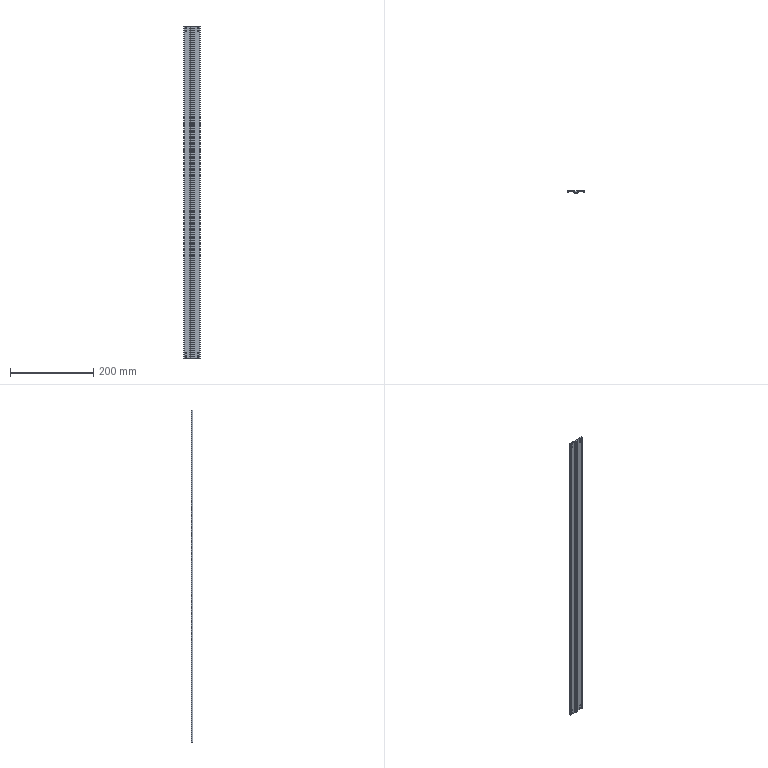Part | STEP file | BODY10_E-RAM6-S-640-ME30-C5 | 1 solid | 38 faces | box 40 x 4.5 x 795.5 mm | volume 67309 mm3 | cylinder 22 | plane 16 | commonest cylinder face diameters 3.4 x8 0.4 x4 0.6 x4 4 x4 2 x2
STEP:
#1=CARTESIAN_POINT('',(-20.,-1.,397.75));
#2=VERTEX_POINT('',#1);
#3=CARTESIAN_POINT('',(-20.,-1.7,397.75));
#4=VERTEX_POINT('',#3);
#5=CARTESIAN_POINT('',(-20.,-2.,397.75));
#6=DIRECTION('',(0.,-1.,0.));
#7=VECTOR('',#6,1000.);
#8=LINE('',#5,#7);
#9=EDGE_CURVE('',#2,#4,#8,.T.);
#10=ORIENTED_EDGE('',*,*,#9,.F.);
#11=CARTESIAN_POINT('',(-20.,-1.,-397.75));
#12=VERTEX_POINT('',#11);
#13=CARTESIAN_POINT('',(-20.,-1.,397.75));
#14=DIRECTION('',(0.,0.,-1.));
#15=VECTOR('',#14,1000.);
#16=LINE('',#13,#15);
#17=EDGE_CURVE('',#2,#12,#16,.T.);
#18=ORIENTED_EDGE('',*,*,#17,.T.);
#19=CARTESIAN_POINT('',(-20.,-1.7,-397.75));
#20=VERTEX_POINT('',#19);
#21=CARTESIAN_POINT('',(-20.,-2.,-397.75));
#22=DIRECTION('',(0.,-1.,0.));
#23=VECTOR('',#22,1000.);
#24=LINE('',#21,#23);
#25=EDGE_CURVE('',#12,#20,#24,.T.);
#26=ORIENTED_EDGE('',*,*,#25,.T.);
#27=CARTESIAN_POINT('',(-20.,-1.7,397.75));
#28=DIRECTION('',(0.,0.,1.));
#29=VECTOR('',#28,1000.);
#30=LINE('',#27,#29);
#31=EDGE_CURVE('',#20,#4,#30,.T.);
#32=ORIENTED_EDGE('',*,*,#31,.T.);
#33=EDGE_LOOP('',(#10,#18,#26,#32));
#34=FACE_OUTER_BOUND('',#33,.T.);
#35=CARTESIAN_POINT('',(-20.,-2.,397.75));
#36=DIRECTION('',(1.,0.,0.));
#37=DIRECTION('',(0.,0.,-1.));
#38=AXIS2_PLACEMENT_3D('',#35,#36,#37);
#39=PLANE('',#38);
#40=ADVANCED_FACE('',(#34),#39,.F.);
#41=CARTESIAN_POINT('',(-19.7,-2.,-397.75));
#42=VERTEX_POINT('',#41);
#43=CARTESIAN_POINT('',(-17.2,-2.,-397.75));
#44=VERTEX_POINT('',#43);
#45=CARTESIAN_POINT('',(-17.,-2.,-397.75));
#46=DIRECTION('',(1.,0.,0.));
#47=VECTOR('',#46,1000.);
#48=LINE('',#45,#47);
#49=EDGE_CURVE('',#42,#44,#48,.T.);
#50=ORIENTED_EDGE('',*,*,#49,.T.);
#51=CARTESIAN_POINT('',(-17.2,-2.,397.75));
#52=VERTEX_POINT('',#51);
#53=CARTESIAN_POINT('',(-17.2,-2.,397.75));
#54=DIRECTION('',(0.,0.,1.));
#55=VECTOR('',#54,1000.);
#56=LINE('',#53,#55);
#57=EDGE_CURVE('',#44,#52,#56,.T.);
#58=ORIENTED_EDGE('',*,*,#57,.T.);
#59=CARTESIAN_POINT('',(-19.7,-2.,397.75));
#60=VERTEX_POINT('',#59);
#61=CARTESIAN_POINT('',(-17.,-2.,397.75));
#62=DIRECTION('',(1.,0.,0.));
#63=VECTOR('',#62,1000.);
#64=LINE('',#61,#63);
#65=EDGE_CURVE('',#60,#52,#64,.T.);
#66=ORIENTED_EDGE('',*,*,#65,.F.);
#67=CARTESIAN_POINT('',(-19.7,-2.,397.75));
#68=DIRECTION('',(0.,0.,-1.));
#69=VECTOR('',#68,1000.);
#70=LINE('',#67,#69);
#71=EDGE_CURVE('',#60,#42,#70,.T.);
#72=ORIENTED_EDGE('',*,*,#71,.T.);
#73=EDGE_LOOP('',(#50,#58,#66,#72));
#74=FACE_OUTER_BOUND('',#73,.T.);
#75=CARTESIAN_POINT('',(-17.,-2.,397.75));
#76=DIRECTION('',(0.,1.,0.));
#77=DIRECTION('',(-1.,0.,0.));
#78=AXIS2_PLACEMENT_3D('',#75,#76,#77);
#79=PLANE('',#78);
#80=ADVANCED_FACE('',(#74),#79,.F.);
#81=CARTESIAN_POINT('',(-17.,-1.8,-397.75));
#82=VERTEX_POINT('',#81);
#83=CARTESIAN_POINT('',(-17.,-1.7,-397.75));
#84=VERTEX_POINT('',#83);
#85=CARTESIAN_POINT('',(-17.,-1.5,-397.75));
#86=DIRECTION('',(0.,1.,0.));
#87=VECTOR('',#86,1000.);
#88=LINE('',#85,#87);
#89=EDGE_CURVE('',#82,#84,#88,.T.);
#90=ORIENTED_EDGE('',*,*,#89,.T.);
#91=CARTESIAN_POINT('',(-17.,-1.7,397.75));
#92=VERTEX_POINT('',#91);
#93=CARTESIAN_POINT('',(-17.,-1.7,397.75));
#94=DIRECTION('',(0.,0.,1.));
#95=VECTOR('',#94,1000.);
#96=LINE('',#93,#95);
#97=EDGE_CURVE('',#84,#92,#96,.T.);
#98=ORIENTED_EDGE('',*,*,#97,.T.);
#99=CARTESIAN_POINT('',(-17.,-1.8,397.75));
#100=VERTEX_POINT('',#99);
#101=CARTESIAN_POINT('',(-17.,-1.5,397.75));
#102=DIRECTION('',(0.,1.,0.));
#103=VECTOR('',#102,1000.);
#104=LINE('',#101,#103);
#105=EDGE_CURVE('',#100,#92,#104,.T.);
#106=ORIENTED_EDGE('',*,*,#105,.F.);
#107=CARTESIAN_POINT('',(-17.,-1.8,397.75));
#108=DIRECTION('',(0.,0.,-1.));
#109=VECTOR('',#108,1000.);
#110=LINE('',#107,#109);
#111=EDGE_CURVE('',#100,#82,#110,.T.);
#112=ORIENTED_EDGE('',*,*,#111,.T.);
#113=EDGE_LOOP('',(#90,#98,#106,#112));
#114=FACE_OUTER_BOUND('',#113,.T.);
#115=CARTESIAN_POINT('',(-17.,-1.5,397.75));
#116=DIRECTION('',(-1.,0.,0.));
#117=DIRECTION('',(0.,0.,1.));
#118=AXIS2_PLACEMENT_3D('',#115,#116,#117);
#119=PLANE('',#118);
#120=ADVANCED_FACE('',(#114),#119,.F.);
#121=CARTESIAN_POINT('',(-16.8,-1.5,397.75));
#122=VERTEX_POINT('',#121);
#123=CARTESIAN_POINT('',(-5.937,-1.5,397.75));
#124=VERTEX_POINT('',#123);
#125=CARTESIAN_POINT('',(-5.,-1.5,397.75));
#126=DIRECTION('',(1.,0.,0.));
#127=VECTOR('',#126,1000.);
#128=LINE('',#125,#127);
#129=EDGE_CURVE('',#122,#124,#128,.T.);
#130=ORIENTED_EDGE('',*,*,#129,.F.);
#131=CARTESIAN_POINT('',(-16.8,-1.5,-397.75));
#132=VERTEX_POINT('',#131);
#133=CARTESIAN_POINT('',(-16.8,-1.5,-397.75));
#134=DIRECTION('',(0.,0.,-1.));
#135=VECTOR('',#134,1000.);
#136=LINE('',#133,#135);
#137=EDGE_CURVE('',#122,#132,#136,.T.);
#138=ORIENTED_EDGE('',*,*,#137,.T.);
#139=CARTESIAN_POINT('',(-5.937,-1.5,-397.75));
#140=VERTEX_POINT('',#139);
#141=CARTESIAN_POINT('',(-5.,-1.5,-397.75));
#142=DIRECTION('',(1.,0.,0.));
#143=VECTOR('',#142,1000.);
#144=LINE('',#141,#143);
#145=EDGE_CURVE('',#132,#140,#144,.T.);
#146=ORIENTED_EDGE('',*,*,#145,.T.);
#147=CARTESIAN_POINT('',(-5.937,-1.5,397.75));
#148=DIRECTION('',(0.,0.,1.));
#149=VECTOR('',#148,1000.);
#150=LINE('',#147,#149);
#151=EDGE_CURVE('',#140,#124,#150,.T.);
#152=ORIENTED_EDGE('',*,*,#151,.T.);
#153=EDGE_LOOP('',(#130,#138,#146,#152));
#154=FACE_OUTER_BOUND('',#153,.T.);
#155=CARTESIAN_POINT('',(-15.7,-1.5,-386.));
#156=VERTEX_POINT('',#155);
#157=CARTESIAN_POINT('',(-14.,-1.5,-387.7));
#158=VERTEX_POINT('',#157);
#159=CARTESIAN_POINT('',(-14.,-1.5,-386.));
#160=DIRECTION('',(0.,-1.,0.));
#161=DIRECTION('',(-1.,0.,0.));
#162=AXIS2_PLACEMENT_3D('',#159,#160,#161);
#163=CIRCLE('',#162,1.7);
#164=EDGE_CURVE('',#156,#158,#163,.T.);
#165=ORIENTED_EDGE('',*,*,#164,.F.);
#166=CARTESIAN_POINT('',(-14.,-1.5,-386.));
#167=DIRECTION('',(0.,-1.,0.));
#168=DIRECTION('',(-1.,0.,0.));
#169=AXIS2_PLACEMENT_3D('',#166,#167,#168);
#170=CIRCLE('',#169,1.7);
#171=EDGE_CURVE('',#158,#156,#170,.T.);
#172=ORIENTED_EDGE('',*,*,#171,.F.);
#173=EDGE_LOOP('',(#165,#172));
#174=FACE_BOUND('',#173,.T.);
#175=CARTESIAN_POINT('',(-15.7,-1.5,-394.));
#176=VERTEX_POINT('',#175);
#177=CARTESIAN_POINT('',(-14.,-1.5,-395.7));
#178=VERTEX_POINT('',#177);
#179=CARTESIAN_POINT('',(-14.,-1.5,-394.));
#180=DIRECTION('',(0.,-1.,0.));
#181=DIRECTION('',(-1.,0.,0.));
#182=AXIS2_PLACEMENT_3D('',#179,#180,#181);
#183=CIRCLE('',#182,1.7);
#184=EDGE_CURVE('',#176,#178,#183,.T.);
#185=ORIENTED_EDGE('',*,*,#184,.F.);
#186=CARTESIAN_POINT('',(-14.,-1.5,-394.));
#187=DIRECTION('',(0.,-1.,0.));
#188=DIRECTION('',(-1.,0.,0.));
#189=AXIS2_PLACEMENT_3D('',#186,#187,#188);
#190=CIRCLE('',#189,1.7);
#191=EDGE_CURVE('',#178,#176,#190,.T.);
#192=ORIENTED_EDGE('',*,*,#191,.F.);
#193=EDGE_LOOP('',(#185,#192));
#194=FACE_BOUND('',#193,.T.);
#195=CARTESIAN_POINT('',(-15.7,-1.5,386.));
#196=VERTEX_POINT('',#195);
#197=CARTESIAN_POINT('',(-14.,-1.5,384.3));
#198=VERTEX_POINT('',#197);
#199=CARTESIAN_POINT('',(-14.,-1.5,386.));
#200=DIRECTION('',(0.,1.,0.));
#201=DIRECTION('',(-1.,0.,0.));
#202=AXIS2_PLACEMENT_3D('',#199,#200,#201);
#203=CIRCLE('',#202,1.7);
#204=EDGE_CURVE('',#196,#198,#203,.T.);
#205=ORIENTED_EDGE('',*,*,#204,.T.);
#206=CARTESIAN_POINT('',(-14.,-1.5,386.));
#207=DIRECTION('',(0.,1.,0.));
#208=DIRECTION('',(-1.,0.,0.));
#209=AXIS2_PLACEMENT_3D('',#206,#207,#208);
#210=CIRCLE('',#209,1.7);
#211=EDGE_CURVE('',#198,#196,#210,.T.);
#212=ORIENTED_EDGE('',*,*,#211,.T.);
#213=EDGE_LOOP('',(#205,#212));
#214=FACE_BOUND('',#213,.T.);
#215=CARTESIAN_POINT('',(-15.7,-1.5,394.));
#216=VERTEX_POINT('',#215);
#217=CARTESIAN_POINT('',(-14.,-1.5,392.3));
#218=VERTEX_POINT('',#217);
#219=CARTESIAN_POINT('',(-14.,-1.5,394.));
#220=DIRECTION('',(0.,1.,0.));
#221=DIRECTION('',(-1.,0.,0.));
#222=AXIS2_PLACEMENT_3D('',#219,#220,#221);
#223=CIRCLE('',#222,1.7);
#224=EDGE_CURVE('',#216,#218,#223,.T.);
#225=ORIENTED_EDGE('',*,*,#224,.T.);
#226=CARTESIAN_POINT('',(-14.,-1.5,394.));
#227=DIRECTION('',(0.,1.,0.));
#228=DIRECTION('',(-1.,0.,0.));
#229=AXIS2_PLACEMENT_3D('',#226,#227,#228);
#230=CIRCLE('',#229,1.7);
#231=EDGE_CURVE('',#218,#216,#230,.T.);
#232=ORIENTED_EDGE('',*,*,#231,.T.);
#233=EDGE_LOOP('',(#225,#232));
#234=FACE_BOUND('',#233,.T.);
#235=CARTESIAN_POINT('',(-5.,-1.5,397.75));
#236=DIRECTION('',(0.,1.,0.));
#237=DIRECTION('',(-1.,0.,0.));
#238=AXIS2_PLACEMENT_3D('',#235,#236,#237);
#239=PLANE('',#238);
#240=ADVANCED_FACE('',(#154,#174,#194,#214,#234),#239,.F.);
#241=CARTESIAN_POINT('',(-4.4,-2.22,-397.75));
#242=VERTEX_POINT('',#241);
#243=CARTESIAN_POINT('',(-3.1,-3.78,-397.75));
#244=VERTEX_POINT('',#243);
#245=CARTESIAN_POINT('',(-2.5,-4.5,-397.75));
#246=DIRECTION('',(0.6402,-0.7682,0.));
#247=VECTOR('',#246,1000.);
#248=LINE('',#245,#247);
#249=EDGE_CURVE('',#242,#244,#248,.T.);
#250=ORIENTED_EDGE('',*,*,#249,.T.);
#251=CARTESIAN_POINT('',(-3.1,-3.78,397.75));
#252=VERTEX_POINT('',#251);
#253=CARTESIAN_POINT('',(-3.1,-3.78,397.75));
#254=DIRECTION('',(0.,0.,1.));
#255=VECTOR('',#254,1000.);
#256=LINE('',#253,#255);
#257=EDGE_CURVE('',#244,#252,#256,.T.);
#258=ORIENTED_EDGE('',*,*,#257,.T.);
#259=CARTESIAN_POINT('',(-4.4,-2.22,397.75));
#260=VERTEX_POINT('',#259);
#261=CARTESIAN_POINT('',(-2.5,-4.5,397.75));
#262=DIRECTION('',(0.6402,-0.7682,0.));
#263=VECTOR('',#262,1000.);
#264=LINE('',#261,#263);
#265=EDGE_CURVE('',#260,#252,#264,.T.);
#266=ORIENTED_EDGE('',*,*,#265,.F.);
#267=CARTESIAN_POINT('',(-4.4,-2.22,-397.75));
#268=DIRECTION('',(0.,0.,-1.));
#269=VECTOR('',#268,1000.);
#270=LINE('',#267,#269);
#271=EDGE_CURVE('',#260,#242,#270,.T.);
#272=ORIENTED_EDGE('',*,*,#271,.T.);
#273=EDGE_LOOP('',(#250,#258,#266,#272));
#274=FACE_OUTER_BOUND('',#273,.T.);
#275=CARTESIAN_POINT('',(-2.5,-4.5,397.75));
#276=DIRECTION('',(0.7682,0.6402,0.));
#277=DIRECTION('',(-0.6402,0.7682,0.));
#278=AXIS2_PLACEMENT_3D('',#275,#276,#277);
#279=PLANE('',#278);
#280=ADVANCED_FACE('',(#274),#279,.F.);
#281=CARTESIAN_POINT('',(-1.563,-4.5,-397.75));
#282=VERTEX_POINT('',#281);
#283=CARTESIAN_POINT('',(1.563,-4.5,-397.75));
#284=VERTEX_POINT('',#283);
#285=CARTESIAN_POINT('',(2.5,-4.5,-397.75));
#286=DIRECTION('',(1.,0.,0.));
#287=VECTOR('',#286,1000.);
#288=LINE('',#285,#287);
#289=EDGE_CURVE('',#282,#284,#288,.T.);
#290=ORIENTED_EDGE('',*,*,#289,.T.);
#291=CARTESIAN_POINT('',(1.563,-4.5,397.75));
#292=VERTEX_POINT('',#291);
#293=CARTESIAN_POINT('',(1.563,-4.5,397.75));
#294=DIRECTION('',(0.,0.,1.));
#295=VECTOR('',#294,1000.);
#296=LINE('',#293,#295);
#297=EDGE_CURVE('',#284,#292,#296,.T.);
#298=ORIENTED_EDGE('',*,*,#297,.T.);
#299=CARTESIAN_POINT('',(-1.563,-4.5,397.75));
#300=VERTEX_POINT('',#299);
#301=CARTESIAN_POINT('',(2.5,-4.5,397.75));
#302=DIRECTION('',(1.,0.,0.));
#303=VECTOR('',#302,1000.);
#304=LINE('',#301,#303);
#305=EDGE_CURVE('',#300,#292,#304,.T.);
#306=ORIENTED_EDGE('',*,*,#305,.F.);
#307=CARTESIAN_POINT('',(-1.563,-4.5,397.75));
#308=DIRECTION('',(0.,0.,-1.));
#309=VECTOR('',#308,1000.);
#310=LINE('',#307,#309);
#311=EDGE_CURVE('',#300,#282,#310,.T.);
#312=ORIENTED_EDGE('',*,*,#311,.T.);
#313=EDGE_LOOP('',(#290,#298,#306,#312));
#314=FACE_OUTER_BOUND('',#313,.T.);
#315=CARTESIAN_POINT('',(2.5,-4.5,397.75));
#316=DIRECTION('',(0.,1.,0.));
#317=DIRECTION('',(0.,0.,1.));
#318=AXIS2_PLACEMENT_3D('',#315,#316,#317);
#319=PLANE('',#318);
#320=ADVANCED_FACE('',(#314),#319,.F.);
#321=CARTESIAN_POINT('',(3.1,-3.78,-397.75));
#322=VERTEX_POINT('',#321);
#323=CARTESIAN_POINT('',(4.4,-2.22,-397.75));
#324=VERTEX_POINT('',#323);
#325=CARTESIAN_POINT('',(5.,-1.5,-397.75));
#326=DIRECTION('',(0.6402,0.7682,0.));
#327=VECTOR('',#326,1000.);
#328=LINE('',#325,#327);
#329=EDGE_CURVE('',#322,#324,#328,.T.);
#330=ORIENTED_EDGE('',*,*,#329,.T.);
#331=CARTESIAN_POINT('',(4.4,-2.22,397.75));
#332=VERTEX_POINT('',#331);
#333=CARTESIAN_POINT('',(4.4,-2.22,397.75));
#334=DIRECTION('',(0.,0.,1.));
#335=VECTOR('',#334,1000.);
#336=LINE('',#333,#335);
#337=EDGE_CURVE('',#324,#332,#336,.T.);
#338=ORIENTED_EDGE('',*,*,#337,.T.);
#339=CARTESIAN_POINT('',(3.1,-3.78,397.75));
#340=VERTEX_POINT('',#339);
#341=CARTESIAN_POINT('',(5.,-1.5,397.75));
#342=DIRECTION('',(0.6402,0.7682,0.));
#343=VECTOR('',#342,1000.);
#344=LINE('',#341,#343);
#345=EDGE_CURVE('',#340,#332,#344,.T.);
#346=ORIENTED_EDGE('',*,*,#345,.F.);
#347=CARTESIAN_POINT('',(3.1,-3.78,397.75));
#348=DIRECTION('',(0.,0.,-1.));
#349=VECTOR('',#348,1000.);
#350=LINE('',#347,#349);
#351=EDGE_CURVE('',#340,#322,#350,.T.);
#352=ORIENTED_EDGE('',*,*,#351,.T.);
#353=EDGE_LOOP('',(#330,#338,#346,#352));
#354=FACE_OUTER_BOUND('',#353,.T.);
#355=CARTESIAN_POINT('',(5.,-1.5,397.75));
#356=DIRECTION('',(-0.7682,0.6402,0.));
#357=DIRECTION('',(-0.6402,-0.7682,0.));
#358=AXIS2_PLACEMENT_3D('',#355,#356,#357);
#359=PLANE('',#358);
#360=ADVANCED_FACE('',(#354),#359,.F.);
#361=CARTESIAN_POINT('',(5.937,-1.5,-397.75));
#362=VERTEX_POINT('',#361);
#363=CARTESIAN_POINT('',(16.8,-1.5,-397.75));
#364=VERTEX_POINT('',#363);
#365=CARTESIAN_POINT('',(17.,-1.5,-397.75));
#366=DIRECTION('',(1.,0.,0.));
#367=VECTOR('',#366,1000.);
#368=LINE('',#365,#367);
#369=EDGE_CURVE('',#362,#364,#368,.T.);
#370=ORIENTED_EDGE('',*,*,#369,.T.);
#371=CARTESIAN_POINT('',(16.8,-1.5,397.75));
#372=VERTEX_POINT('',#371);
#373=CARTESIAN_POINT('',(16.8,-1.5,397.75));
#374=DIRECTION('',(0.,0.,1.));
#375=VECTOR('',#374,1000.);
#376=LINE('',#373,#375);
#377=EDGE_CURVE('',#364,#372,#376,.T.);
#378=ORIENTED_EDGE('',*,*,#377,.T.);
#379=CARTESIAN_POINT('',(5.937,-1.5,397.75));
#380=VERTEX_POINT('',#379);
#381=CARTESIAN_POINT('',(17.,-1.5,397.75));
#382=DIRECTION('',(1.,0.,0.));
#383=VECTOR('',#382,1000.);
#384=LINE('',#381,#383);
#385=EDGE_CURVE('',#380,#372,#384,.T.);
#386=ORIENTED_EDGE('',*,*,#385,.F.);
#387=CARTESIAN_POINT('',(5.937,-1.5,-397.75));
#388=DIRECTION('',(0.,0.,-1.));
#389=VECTOR('',#388,1000.);
#390=LINE('',#387,#389);
#391=EDGE_CURVE('',#380,#362,#390,.T.);
#392=ORIENTED_EDGE('',*,*,#391,.T.);
#393=EDGE_LOOP('',(#370,#378,#386,#392));
#394=FACE_OUTER_BOUND('',#393,.T.);
#395=CARTESIAN_POINT('',(12.3,-1.5,-386.));
#396=VERTEX_POINT('',#395);
#397=CARTESIAN_POINT('',(14.,-1.5,-387.7));
#398=VERTEX_POINT('',#397);
#399=CARTESIAN_POINT('',(14.,-1.5,-386.));
#400=DIRECTION('',(0.,-1.,0.));
#401=DIRECTION('',(-1.,0.,0.));
#402=AXIS2_PLACEMENT_3D('',#399,#400,#401);
#403=CIRCLE('',#402,1.7);
#404=EDGE_CURVE('',#396,#398,#403,.T.);
#405=ORIENTED_EDGE('',*,*,#404,.F.);
#406=CARTESIAN_POINT('',(14.,-1.5,-386.));
#407=DIRECTION('',(0.,-1.,0.));
#408=DIRECTION('',(-1.,0.,0.));
#409=AXIS2_PLACEMENT_3D('',#406,#407,#408);
#410=CIRCLE('',#409,1.7);
#411=EDGE_CURVE('',#398,#396,#410,.T.);
#412=ORIENTED_EDGE('',*,*,#411,.F.);
#413=EDGE_LOOP('',(#405,#412));
#414=FACE_BOUND('',#413,.T.);
#415=CARTESIAN_POINT('',(12.3,-1.5,-394.));
#416=VERTEX_POINT('',#415);
#417=CARTESIAN_POINT('',(14.,-1.5,-395.7));
#418=VERTEX_POINT('',#417);
#419=CARTESIAN_POINT('',(14.,-1.5,-394.));
#420=DIRECTION('',(0.,-1.,0.));
#421=DIRECTION('',(-1.,0.,0.));
#422=AXIS2_PLACEMENT_3D('',#419,#420,#421);
#423=CIRCLE('',#422,1.7);
#424=EDGE_CURVE('',#416,#418,#423,.T.);
#425=ORIENTED_EDGE('',*,*,#424,.F.);
#426=CARTESIAN_POINT('',(14.,-1.5,-394.));
#427=DIRECTION('',(0.,-1.,0.));
#428=DIRECTION('',(-1.,0.,0.));
#429=AXIS2_PLACEMENT_3D('',#426,#427,#428);
#430=CIRCLE('',#429,1.7);
#431=EDGE_CURVE('',#418,#416,#430,.T.);
#432=ORIENTED_EDGE('',*,*,#431,.F.);
#433=EDGE_LOOP('',(#425,#432));
#434=FACE_BOUND('',#433,.T.);
#435=CARTESIAN_POINT('',(12.3,-1.5,386.));
#436=VERTEX_POINT('',#435);
#437=CARTESIAN_POINT('',(14.,-1.5,384.3));
#438=VERTEX_POINT('',#437);
#439=CARTESIAN_POINT('',(14.,-1.5,386.));
#440=DIRECTION('',(0.,1.,0.));
#441=DIRECTION('',(-1.,0.,0.));
#442=AXIS2_PLACEMENT_3D('',#439,#440,#441);
#443=CIRCLE('',#442,1.7);
#444=EDGE_CURVE('',#436,#438,#443,.T.);
#445=ORIENTED_EDGE('',*,*,#444,.T.);
#446=CARTESIAN_POINT('',(14.,-1.5,386.));
#447=DIRECTION('',(0.,1.,0.));
#448=DIRECTION('',(-1.,0.,0.));
#449=AXIS2_PLACEMENT_3D('',#446,#447,#448);
#450=CIRCLE('',#449,1.7);
#451=EDGE_CURVE('',#438,#436,#450,.T.);
#452=ORIENTED_EDGE('',*,*,#451,.T.);
#453=EDGE_LOOP('',(#445,#452));
#454=FACE_BOUND('',#453,.T.);
#455=CARTESIAN_POINT('',(12.3,-1.5,394.));
#456=VERTEX_POINT('',#455);
#457=CARTESIAN_POINT('',(14.,-1.5,392.3));
#458=VERTEX_POINT('',#457);
#459=CARTESIAN_POINT('',(14.,-1.5,394.));
#460=DIRECTION('',(0.,1.,0.));
#461=DIRECTION('',(-1.,0.,0.));
#462=AXIS2_PLACEMENT_3D('',#459,#460,#461);
#463=CIRCLE('',#462,1.7);
#464=EDGE_CURVE('',#456,#458,#463,.T.);
#465=ORIENTED_EDGE('',*,*,#464,.T.);
#466=CARTESIAN_POINT('',(14.,-1.5,394.));
#467=DIRECTION('',(0.,1.,0.));
#468=DIRECTION('',(-1.,0.,0.));
#469=AXIS2_PLACEMENT_3D('',#466,#467,#468);
#470=CIRCLE('',#469,1.7);
#471=EDGE_CURVE('',#458,#456,#470,.T.);
#472=ORIENTED_EDGE('',*,*,#471,.T.);
#473=EDGE_LOOP('',(#465,#472));
#474=FACE_BOUND('',#473,.T.);
#475=CARTESIAN_POINT('',(17.,-1.5,397.75));
#476=DIRECTION('',(0.,1.,0.));
#477=DIRECTION('',(-1.,0.,0.));
#478=AXIS2_PLACEMENT_3D('',#475,#476,#477);
#479=PLANE('',#478);
#480=ADVANCED_FACE('',(#394,#414,#434,#454,#474),#479,.F.);
#481=CARTESIAN_POINT('',(17.,-1.7,397.75));
#482=VERTEX_POINT('',#481);
#483=CARTESIAN_POINT('',(17.,-1.8,397.75));
#484=VERTEX_POINT('',#483);
#485=CARTESIAN_POINT('',(17.,-2.,397.75));
#486=DIRECTION('',(0.,-1.,0.));
#487=VECTOR('',#486,1000.);
#488=LINE('',#485,#487);
#489=EDGE_CURVE('',#482,#484,#488,.T.);
#490=ORIENTED_EDGE('',*,*,#489,.F.);
#491=CARTESIAN_POINT('',(17.,-1.7,-397.75));
#492=VERTEX_POINT('',#491);
#493=CARTESIAN_POINT('',(17.,-1.7,-397.75));
#494=DIRECTION('',(0.,0.,-1.));
#495=VECTOR('',#494,1000.);
#496=LINE('',#493,#495);
#497=EDGE_CURVE('',#482,#492,#496,.T.);
#498=ORIENTED_EDGE('',*,*,#497,.T.);
#499=CARTESIAN_POINT('',(17.,-1.8,-397.75));
#500=VERTEX_POINT('',#499);
#501=CARTESIAN_POINT('',(17.,-2.,-397.75));
#502=DIRECTION('',(0.,-1.,0.));
#503=VECTOR('',#502,1000.);
#504=LINE('',#501,#503);
#505=EDGE_CURVE('',#492,#500,#504,.T.);
#506=ORIENTED_EDGE('',*,*,#505,.T.);
#507=CARTESIAN_POINT('',(17.,-1.8,397.75));
#508=DIRECTION('',(0.,0.,1.));
#509=VECTOR('',#508,1000.);
#510=LINE('',#507,#509);
#511=EDGE_CURVE('',#500,#484,#510,.T.);
#512=ORIENTED_EDGE('',*,*,#511,.T.);
#513=EDGE_LOOP('',(#490,#498,#506,#512));
#514=FACE_OUTER_BOUND('',#513,.T.);
#515=CARTESIAN_POINT('',(17.,-2.,397.75));
#516=DIRECTION('',(1.,0.,0.));
#517=DIRECTION('',(0.,0.,-1.));
#518=AXIS2_PLACEMENT_3D('',#515,#516,#517);
#519=PLANE('',#518);
#520=ADVANCED_FACE('',(#514),#519,.F.);
#521=CARTESIAN_POINT('',(17.2,-2.,397.75));
#522=VERTEX_POINT('',#521);
#523=CARTESIAN_POINT('',(19.7,-2.,397.75));
#524=VERTEX_POINT('',#523);
#525=CARTESIAN_POINT('',(20.,-2.,397.75));
#526=DIRECTION('',(1.,0.,0.));
#527=VECTOR('',#526,1000.);
#528=LINE('',#525,#527);
#529=EDGE_CURVE('',#522,#524,#528,.T.);
#530=ORIENTED_EDGE('',*,*,#529,.F.);
#531=CARTESIAN_POINT('',(17.2,-2.,-397.75));
#532=VERTEX_POINT('',#531);
#533=CARTESIAN_POINT('',(17.2,-2.,397.75));
#534=DIRECTION('',(0.,0.,-1.));
#535=VECTOR('',#534,1000.);
#536=LINE('',#533,#535);
#537=EDGE_CURVE('',#522,#532,#536,.T.);
#538=ORIENTED_EDGE('',*,*,#537,.T.);
#539=CARTESIAN_POINT('',(19.7,-2.,-397.75));
#540=VERTEX_POINT('',#539);
#541=CARTESIAN_POINT('',(20.,-2.,-397.75));
#542=DIRECTION('',(1.,0.,0.));
#543=VECTOR('',#542,1000.);
#544=LINE('',#541,#543);
#545=EDGE_CURVE('',#532,#540,#544,.T.);
#546=ORIENTED_EDGE('',*,*,#545,.T.);
#547=CARTESIAN_POINT('',(19.7,-2.,397.75));
#548=DIRECTION('',(0.,0.,1.));
#549=VECTOR('',#548,1000.);
#550=LINE('',#547,#549);
#551=EDGE_CURVE('',#540,#524,#550,.T.);
#552=ORIENTED_EDGE('',*,*,#551,.T.);
#553=EDGE_LOOP('',(#530,#538,#546,#552));
#554=FACE_OUTER_BOUND('',#553,.T.);
#555=CARTESIAN_POINT('',(20.,-2.,397.75));
#556=DIRECTION('',(0.,1.,0.));
#557=DIRECTION('',(-1.,0.,0.));
#558=AXIS2_PLACEMENT_3D('',#555,#556,#557);
#559=PLANE('',#558);
#560=ADVANCED_FACE('',(#554),#559,.F.);
#561=CARTESIAN_POINT('',(20.,-1.7,-397.75));
#562=VERTEX_POINT('',#561);
#563=CARTESIAN_POINT('',(20.,-1.,-397.75));
#564=VERTEX_POINT('',#563);
#565=CARTESIAN_POINT('',(20.,0.,-397.75));
#566=DIRECTION('',(0.,1.,0.));
#567=VECTOR('',#566,1000.);
#568=LINE('',#565,#567);
#569=EDGE_CURVE('',#562,#564,#568,.T.);
#570=ORIENTED_EDGE('',*,*,#569,.T.);
#571=CARTESIAN_POINT('',(20.,-1.,397.75));
#572=VERTEX_POINT('',#571);
#573=CARTESIAN_POINT('',(20.,-1.,397.75));
#574=DIRECTION('',(0.,0.,1.));
#575=VECTOR('',#574,1000.);
#576=LINE('',#573,#575);
#577=EDGE_CURVE('',#564,#572,#576,.T.);
#578=ORIENTED_EDGE('',*,*,#577,.T.);
#579=CARTESIAN_POINT('',(20.,-1.7,397.75));
#580=VERTEX_POINT('',#579);
#581=CARTESIAN_POINT('',(20.,0.,397.75));
#582=DIRECTION('',(0.,1.,0.));
#583=VECTOR('',#582,1000.);
#584=LINE('',#581,#583);
#585=EDGE_CURVE('',#580,#572,#584,.T.);
#586=ORIENTED_EDGE('',*,*,#585,.F.);
#587=CARTESIAN_POINT('',(20.,-1.7,397.75));
#588=DIRECTION('',(0.,0.,-1.));
#589=VECTOR('',#588,1000.);
#590=LINE('',#587,#589);
#591=EDGE_CURVE('',#580,#562,#590,.T.);
#592=ORIENTED_EDGE('',*,*,#591,.T.);
#593=EDGE_LOOP('',(#570,#578,#586,#592));
#594=FACE_OUTER_BOUND('',#593,.T.);
#595=CARTESIAN_POINT('',(20.,0.,397.75));
#596=DIRECTION('',(-1.,0.,0.));
#597=DIRECTION('',(0.,0.,1.));
#598=AXIS2_PLACEMENT_3D('',#595,#596,#597);
#599=PLANE('',#598);
#600=ADVANCED_FACE('',(#594),#599,.F.);
#601=CARTESIAN_POINT('',(19.,0.,397.75));
#602=VERTEX_POINT('',#601);
#603=CARTESIAN_POINT('',(10.3,0.,397.75));
#604=VERTEX_POINT('',#603);
#605=CARTESIAN_POINT('',(10.3,0.,397.75));
#606=DIRECTION('',(-1.,0.,0.));
#607=VECTOR('',#606,1000.);
#608=LINE('',#605,#607);
#609=EDGE_CURVE('',#602,#604,#608,.T.);
#610=ORIENTED_EDGE('',*,*,#609,.F.);
#611=CARTESIAN_POINT('',(19.,0.,-397.75));
#612=VERTEX_POINT('',#611);
#613=CARTESIAN_POINT('',(19.,0.,397.75));
#614=DIRECTION('',(0.,0.,-1.));
#615=VECTOR('',#614,1000.);
#616=LINE('',#613,#615);
#617=EDGE_CURVE('',#602,#612,#616,.T.);
#618=ORIENTED_EDGE('',*,*,#617,.T.);
#619=CARTESIAN_POINT('',(10.3,0.,-397.75));
#620=VERTEX_POINT('',#619);
#621=CARTESIAN_POINT('',(10.3,0.,-397.75));
#622=DIRECTION('',(-1.,0.,0.));
#623=VECTOR('',#622,1000.);
#624=LINE('',#621,#623);
#625=EDGE_CURVE('',#612,#620,#624,.T.);
#626=ORIENTED_EDGE('',*,*,#625,.T.);
#627=CARTESIAN_POINT('',(10.3,0.,397.75));
#628=DIRECTION('',(0.,0.,-1.));
#629=VECTOR('',#628,1000.);
#630=LINE('',#627,#629);
#631=EDGE_CURVE('',#604,#620,#630,.T.);
#632=ORIENTED_EDGE('',*,*,#631,.F.);
#633=EDGE_LOOP('',(#610,#618,#626,#632));
#634=FACE_OUTER_BOUND('',#633,.T.);
#635=CARTESIAN_POINT('',(14.,0.,-387.7));
#636=VERTEX_POINT('',#635);
#637=CARTESIAN_POINT('',(14.,0.,-386.));
#638=DIRECTION('',(0.,-1.,0.));
#639=DIRECTION('',(0.,0.,-1.));
#640=AXIS2_PLACEMENT_3D('',#637,#638,#639);
#641=CIRCLE('',#640,1.7);
#642=EDGE_CURVE('',#636,#636,#641,.T.);
#643=ORIENTED_EDGE('',*,*,#642,.T.);
#644=EDGE_LOOP('',(#643));
#645=FACE_BOUND('',#644,.T.);
#646=CARTESIAN_POINT('',(14.,0.,-395.7));
#647=VERTEX_POINT('',#646);
#648=CARTESIAN_POINT('',(14.,0.,-394.));
#649=DIRECTION('',(0.,-1.,0.));
#650=DIRECTION('',(0.,0.,-1.));
#651=AXIS2_PLACEMENT_3D('',#648,#649,#650);
#652=CIRCLE('',#651,1.7);
#653=EDGE_CURVE('',#647,#647,#652,.T.);
#654=ORIENTED_EDGE('',*,*,#653,.T.);
#655=EDGE_LOOP('',(#654));
#656=FACE_BOUND('',#655,.T.);
#657=CARTESIAN_POINT('',(14.,0.,387.7));
#658=VERTEX_POINT('',#657);
#659=CARTESIAN_POINT('',(14.,0.,384.3));
#660=VERTEX_POINT('',#659);
#661=CARTESIAN_POINT('',(14.,0.,386.));
#662=DIRECTION('',(0.,1.,0.));
#663=DIRECTION('',(0.,0.,1.));
#664=AXIS2_PLACEMENT_3D('',#661,#662,#663);
#665=CIRCLE('',#664,1.7);
#666=EDGE_CURVE('',#658,#660,#665,.T.);
#667=ORIENTED_EDGE('',*,*,#666,.F.);
#668=CARTESIAN_POINT('',(14.,0.,386.));
#669=DIRECTION('',(0.,1.,0.));
#670=DIRECTION('',(0.,0.,1.));
#671=AXIS2_PLACEMENT_3D('',#668,#669,#670);
#672=CIRCLE('',#671,1.7);
#673=EDGE_CURVE('',#660,#658,#672,.T.);
#674=ORIENTED_EDGE('',*,*,#673,.F.);
#675=EDGE_LOOP('',(#667,#674));
#676=FACE_BOUND('',#675,.T.);
#677=CARTESIAN_POINT('',(14.,0.,395.7));
#678=VERTEX_POINT('',#677);
#679=CARTESIAN_POINT('',(14.,0.,392.3));
#680=VERTEX_POINT('',#679);
#681=CARTESIAN_POINT('',(14.,0.,394.));
#682=DIRECTION('',(0.,1.,0.));
#683=DIRECTION('',(0.,0.,1.));
#684=AXIS2_PLACEMENT_3D('',#681,#682,#683);
#685=CIRCLE('',#684,1.7);
#686=EDGE_CURVE('',#678,#680,#685,.T.);
#687=ORIENTED_EDGE('',*,*,#686,.F.);
#688=CARTESIAN_POINT('',(14.,0.,394.));
#689=DIRECTION('',(0.,1.,0.));
#690=DIRECTION('',(0.,0.,1.));
#691=AXIS2_PLACEMENT_3D('',#688,#689,#690);
#692=CIRCLE('',#691,1.7);
#693=EDGE_CURVE('',#680,#678,#692,.T.);
#694=ORIENTED_EDGE('',*,*,#693,.F.);
#695=EDGE_LOOP('',(#687,#694));
#696=FACE_BOUND('',#695,.T.);
#697=CARTESIAN_POINT('',(10.3,0.,397.75));
#698=DIRECTION('',(0.,-1.,0.));
#699=DIRECTION('',(0.,0.,-1.));
#700=AXIS2_PLACEMENT_3D('',#697,#698,#699);
#701=PLANE('',#700);
#702=ADVANCED_FACE('',(#634,#645,#656,#676,#696),#701,.F.);
#703=CARTESIAN_POINT('',(9.7,0.,-397.75));
#704=VERTEX_POINT('',#703);
#705=CARTESIAN_POINT('',(10.,0.,-397.75));
#706=DIRECTION('',(0.,0.,-1.));
#707=DIRECTION('',(1.,0.,0.));
#708=AXIS2_PLACEMENT_3D('',#705,#706,#707);
#709=CIRCLE('',#708,0.3);
#710=EDGE_CURVE('',#620,#704,#709,.T.);
#711=ORIENTED_EDGE('',*,*,#710,.T.);
#712=CARTESIAN_POINT('',(9.7,0.,397.75));
#713=VERTEX_POINT('',#712);
#714=CARTESIAN_POINT('',(9.7,0.,397.75));
#715=DIRECTION('',(0.,0.,-1.));
#716=VECTOR('',#715,1000.);
#717=LINE('',#714,#716);
#718=EDGE_CURVE('',#713,#704,#717,.T.);
#719=ORIENTED_EDGE('',*,*,#718,.F.);
#720=CARTESIAN_POINT('',(10.,0.,397.75));
#721=DIRECTION('',(0.,0.,-1.));
#722=DIRECTION('',(1.,0.,0.));
#723=AXIS2_PLACEMENT_3D('',#720,#721,#722);
#724=CIRCLE('',#723,0.3);
#725=EDGE_CURVE('',#604,#713,#724,.T.);
#726=ORIENTED_EDGE('',*,*,#725,.F.);
#727=ORIENTED_EDGE('',*,*,#631,.T.);
#728=EDGE_LOOP('',(#711,#719,#726,#727));
#729=FACE_OUTER_BOUND('',#728,.T.);
#730=CARTESIAN_POINT('',(10.,0.,397.75));
#731=DIRECTION('',(0.,0.,-1.));
#732=DIRECTION('',(-1.,0.,0.));
#733=AXIS2_PLACEMENT_3D('',#730,#731,#732);
#734=CYLINDRICAL_SURFACE('',#733,0.3);
#735=ADVANCED_FACE('',(#729),#734,.F.);
#736=CARTESIAN_POINT('',(-9.7,0.,-397.75));
#737=VERTEX_POINT('',#736);
#738=CARTESIAN_POINT('',(-9.7,0.,-397.75));
#739=DIRECTION('',(-1.,0.,0.));
#740=VECTOR('',#739,1000.);
#741=LINE('',#738,#740);
#742=EDGE_CURVE('',#704,#737,#741,.T.);
#743=ORIENTED_EDGE('',*,*,#742,.T.);
#744=CARTESIAN_POINT('',(-9.7,0.,397.75));
#745=VERTEX_POINT('',#744);
#746=CARTESIAN_POINT('',(-9.7,0.,397.75));
#747=DIRECTION('',(0.,0.,-1.));
#748=VECTOR('',#747,1000.);
#749=LINE('',#746,#748);
#750=EDGE_CURVE('',#745,#737,#749,.T.);
#751=ORIENTED_EDGE('',*,*,#750,.F.);
#752=CARTESIAN_POINT('',(-9.7,0.,397.75));
#753=DIRECTION('',(-1.,0.,0.));
#754=VECTOR('',#753,1000.);
#755=LINE('',#752,#754);
#756=EDGE_CURVE('',#713,#745,#755,.T.);
#757=ORIENTED_EDGE('',*,*,#756,.F.);
#758=ORIENTED_EDGE('',*,*,#718,.T.);
#759=EDGE_LOOP('',(#743,#751,#757,#758));
#760=FACE_OUTER_BOUND('',#759,.T.);
#761=CARTESIAN_POINT('',(-9.7,0.,397.75));
#762=DIRECTION('',(0.,-1.,0.));
#763=DIRECTION('',(0.,0.,-1.));
#764=AXIS2_PLACEMENT_3D('',#761,#762,#763);
#765=PLANE('',#764);
#766=ADVANCED_FACE('',(#760),#765,.F.);
#767=CARTESIAN_POINT('',(-10.3,0.,-397.75));
#768=VERTEX_POINT('',#767);
#769=CARTESIAN_POINT('',(-10.,0.,-397.75));
#770=DIRECTION('',(0.,0.,-1.));
#771=DIRECTION('',(1.,0.,0.));
#772=AXIS2_PLACEMENT_3D('',#769,#770,#771);
#773=CIRCLE('',#772,0.3);
#774=EDGE_CURVE('',#737,#768,#773,.T.);
#775=ORIENTED_EDGE('',*,*,#774,.T.);
#776=CARTESIAN_POINT('',(-10.3,0.,397.75));
#777=VERTEX_POINT('',#776);
#778=CARTESIAN_POINT('',(-10.3,0.,397.75));
#779=DIRECTION('',(0.,0.,-1.));
#780=VECTOR('',#779,1000.);
#781=LINE('',#778,#780);
#782=EDGE_CURVE('',#777,#768,#781,.T.);
#783=ORIENTED_EDGE('',*,*,#782,.F.);
#784=CARTESIAN_POINT('',(-10.,0.,397.75));
#785=DIRECTION('',(0.,0.,-1.));
#786=DIRECTION('',(1.,0.,0.));
#787=AXIS2_PLACEMENT_3D('',#784,#785,#786);
#788=CIRCLE('',#787,0.3);
#789=EDGE_CURVE('',#745,#777,#788,.T.);
#790=ORIENTED_EDGE('',*,*,#789,.F.);
#791=ORIENTED_EDGE('',*,*,#750,.T.);
#792=EDGE_LOOP('',(#775,#783,#790,#791));
#793=FACE_OUTER_BOUND('',#792,.T.);
#794=CARTESIAN_POINT('',(-10.,0.,397.75));
#795=DIRECTION('',(0.,0.,-1.));
#796=DIRECTION('',(-1.,0.,0.));
#797=AXIS2_PLACEMENT_3D('',#794,#795,#796);
#798=CYLINDRICAL_SURFACE('',#797,0.3);
#799=ADVANCED_FACE('',(#793),#798,.F.);
#800=CARTESIAN_POINT('',(-19.,0.,-397.75));
#801=VERTEX_POINT('',#800);
#802=CARTESIAN_POINT('',(-20.,0.,-397.75));
#803=DIRECTION('',(-1.,0.,0.));
#804=VECTOR('',#803,1000.);
#805=LINE('',#802,#804);
#806=EDGE_CURVE('',#768,#801,#805,.T.);
#807=ORIENTED_EDGE('',*,*,#806,.T.);
#808=CARTESIAN_POINT('',(-19.,0.,397.75));
#809=VERTEX_POINT('',#808);
#810=CARTESIAN_POINT('',(-19.,0.,397.75));
#811=DIRECTION('',(0.,0.,1.));
#812=VECTOR('',#811,1000.);
#813=LINE('',#810,#812);
#814=EDGE_CURVE('',#801,#809,#813,.T.);
#815=ORIENTED_EDGE('',*,*,#814,.T.);
#816=CARTESIAN_POINT('',(-20.,0.,397.75));
#817=DIRECTION('',(-1.,0.,0.));
#818=VECTOR('',#817,1000.);
#819=LINE('',#816,#818);
#820=EDGE_CURVE('',#777,#809,#819,.T.);
#821=ORIENTED_EDGE('',*,*,#820,.F.);
#822=ORIENTED_EDGE('',*,*,#782,.T.);
#823=EDGE_LOOP('',(#807,#815,#821,#822));
#824=FACE_OUTER_BOUND('',#823,.T.);
#825=CARTESIAN_POINT('',(-14.,0.,-387.7));
#826=VERTEX_POINT('',#825);
#827=CARTESIAN_POINT('',(-14.,0.,-386.));
#828=DIRECTION('',(0.,-1.,0.));
#829=DIRECTION('',(0.,0.,-1.));
#830=AXIS2_PLACEMENT_3D('',#827,#828,#829);
#831=CIRCLE('',#830,1.7);
#832=EDGE_CURVE('',#826,#826,#831,.T.);
#833=ORIENTED_EDGE('',*,*,#832,.T.);
#834=EDGE_LOOP('',(#833));
#835=FACE_BOUND('',#834,.T.);
#836=CARTESIAN_POINT('',(-14.,0.,-395.7));
#837=VERTEX_POINT('',#836);
#838=CARTESIAN_POINT('',(-14.,0.,-394.));
#839=DIRECTION('',(0.,-1.,0.));
#840=DIRECTION('',(0.,0.,-1.));
#841=AXIS2_PLACEMENT_3D('',#838,#839,#840);
#842=CIRCLE('',#841,1.7);
#843=EDGE_CURVE('',#837,#837,#842,.T.);
#844=ORIENTED_EDGE('',*,*,#843,.T.);
#845=EDGE_LOOP('',(#844));
#846=FACE_BOUND('',#845,.T.);
#847=CARTESIAN_POINT('',(-14.,0.,387.7));
#848=VERTEX_POINT('',#847);
#849=CARTESIAN_POINT('',(-14.,0.,384.3));
#850=VERTEX_POINT('',#849);
#851=CARTESIAN_POINT('',(-14.,0.,386.));
#852=DIRECTION('',(0.,1.,0.));
#853=DIRECTION('',(0.,0.,1.));
#854=AXIS2_PLACEMENT_3D('',#851,#852,#853);
#855=CIRCLE('',#854,1.7);
#856=EDGE_CURVE('',#848,#850,#855,.T.);
#857=ORIENTED_EDGE('',*,*,#856,.F.);
#858=CARTESIAN_POINT('',(-14.,0.,386.));
#859=DIRECTION('',(0.,1.,0.));
#860=DIRECTION('',(0.,0.,1.));
#861=AXIS2_PLACEMENT_3D('',#858,#859,#860);
#862=CIRCLE('',#861,1.7);
#863=EDGE_CURVE('',#850,#848,#862,.T.);
#864=ORIENTED_EDGE('',*,*,#863,.F.);
#865=EDGE_LOOP('',(#857,#864));
#866=FACE_BOUND('',#865,.T.);
#867=CARTESIAN_POINT('',(-14.,0.,395.7));
#868=VERTEX_POINT('',#867);
#869=CARTESIAN_POINT('',(-14.,0.,392.3));
#870=VERTEX_POINT('',#869);
#871=CARTESIAN_POINT('',(-14.,0.,394.));
#872=DIRECTION('',(0.,1.,0.));
#873=DIRECTION('',(0.,0.,1.));
#874=AXIS2_PLACEMENT_3D('',#871,#872,#873);
#875=CIRCLE('',#874,1.7);
#876=EDGE_CURVE('',#868,#870,#875,.T.);
#877=ORIENTED_EDGE('',*,*,#876,.F.);
#878=CARTESIAN_POINT('',(-14.,0.,394.));
#879=DIRECTION('',(0.,1.,0.));
#880=DIRECTION('',(0.,0.,1.));
#881=AXIS2_PLACEMENT_3D('',#878,#879,#880);
#882=CIRCLE('',#881,1.7);
#883=EDGE_CURVE('',#870,#868,#882,.T.);
#884=ORIENTED_EDGE('',*,*,#883,.F.);
#885=EDGE_LOOP('',(#877,#884));
#886=FACE_BOUND('',#885,.T.);
#887=CARTESIAN_POINT('',(-20.,0.,397.75));
#888=DIRECTION('',(0.,-1.,0.));
#889=DIRECTION('',(0.,0.,-1.));
#890=AXIS2_PLACEMENT_3D('',#887,#888,#889);
#891=PLANE('',#890);
#892=ADVANCED_FACE('',(#824,#835,#846,#866,#886),#891,.F.);
#893=ORIENTED_EDGE('',*,*,#585,.T.);
#894=CARTESIAN_POINT('',(19.,-1.,397.75));
#895=DIRECTION('',(0.,0.,1.));
#896=DIRECTION('',(1.,0.,0.));
#897=AXIS2_PLACEMENT_3D('',#894,#895,#896);
#898=CIRCLE('',#897,1.);
#899=EDGE_CURVE('',#572,#602,#898,.T.);
#900=ORIENTED_EDGE('',*,*,#899,.T.);
#901=ORIENTED_EDGE('',*,*,#609,.T.);
#902=ORIENTED_EDGE('',*,*,#725,.T.);
#903=ORIENTED_EDGE('',*,*,#756,.T.);
#904=ORIENTED_EDGE('',*,*,#789,.T.);
#905=ORIENTED_EDGE('',*,*,#820,.T.);
#906=CARTESIAN_POINT('',(-19.,-1.,397.75));
#907=DIRECTION('',(0.,0.,1.));
#908=DIRECTION('',(1.,0.,0.));
#909=AXIS2_PLACEMENT_3D('',#906,#907,#908);
#910=CIRCLE('',#909,1.);
#911=EDGE_CURVE('',#809,#2,#910,.T.);
#912=ORIENTED_EDGE('',*,*,#911,.T.);
#913=ORIENTED_EDGE('',*,*,#9,.T.);
#914=CARTESIAN_POINT('',(-19.7,-1.7,397.75));
#915=DIRECTION('',(0.,0.,1.));
#916=DIRECTION('',(1.,0.,0.));
#917=AXIS2_PLACEMENT_3D('',#914,#915,#916);
#918=CIRCLE('',#917,0.3);
#919=EDGE_CURVE('',#4,#60,#918,.T.);
#920=ORIENTED_EDGE('',*,*,#919,.T.);
#921=ORIENTED_EDGE('',*,*,#65,.T.);
#922=CARTESIAN_POINT('',(-17.2,-1.8,397.75));
#923=DIRECTION('',(0.,0.,1.));
#924=DIRECTION('',(1.,0.,0.));
#925=AXIS2_PLACEMENT_3D('',#922,#923,#924);
#926=CIRCLE('',#925,0.2);
#927=EDGE_CURVE('',#52,#100,#926,.T.);
#928=ORIENTED_EDGE('',*,*,#927,.T.);
#929=ORIENTED_EDGE('',*,*,#105,.T.);
#930=CARTESIAN_POINT('',(-16.8,-1.7,397.75));
#931=DIRECTION('',(0.,0.,-1.));
#932=DIRECTION('',(1.,0.,0.));
#933=AXIS2_PLACEMENT_3D('',#930,#931,#932);
#934=CIRCLE('',#933,0.2);
#935=EDGE_CURVE('',#92,#122,#934,.T.);
#936=ORIENTED_EDGE('',*,*,#935,.T.);
#937=ORIENTED_EDGE('',*,*,#129,.T.);
#938=CARTESIAN_POINT('',(-5.937,-3.5,397.75));
#939=DIRECTION('',(0.,0.,-1.));
#940=DIRECTION('',(1.,0.,0.));
#941=AXIS2_PLACEMENT_3D('',#938,#939,#940);
#942=CIRCLE('',#941,2.);
#943=EDGE_CURVE('',#124,#260,#942,.T.);
#944=ORIENTED_EDGE('',*,*,#943,.T.);
#945=ORIENTED_EDGE('',*,*,#265,.T.);
#946=CARTESIAN_POINT('',(-1.563,-2.5,397.75));
#947=DIRECTION('',(0.,0.,1.));
#948=DIRECTION('',(1.,0.,0.));
#949=AXIS2_PLACEMENT_3D('',#946,#947,#948);
#950=CIRCLE('',#949,2.);
#951=EDGE_CURVE('',#252,#300,#950,.T.);
#952=ORIENTED_EDGE('',*,*,#951,.T.);
#953=ORIENTED_EDGE('',*,*,#305,.T.);
#954=CARTESIAN_POINT('',(1.563,-2.5,397.75));
#955=DIRECTION('',(0.,0.,1.));
#956=DIRECTION('',(1.,0.,0.));
#957=AXIS2_PLACEMENT_3D('',#954,#955,#956);
#958=CIRCLE('',#957,2.);
#959=EDGE_CURVE('',#292,#340,#958,.T.);
#960=ORIENTED_EDGE('',*,*,#959,.T.);
#961=ORIENTED_EDGE('',*,*,#345,.T.);
#962=CARTESIAN_POINT('',(5.937,-3.5,397.75));
#963=DIRECTION('',(0.,0.,-1.));
#964=DIRECTION('',(1.,0.,0.));
#965=AXIS2_PLACEMENT_3D('',#962,#963,#964);
#966=CIRCLE('',#965,2.);
#967=EDGE_CURVE('',#332,#380,#966,.T.);
#968=ORIENTED_EDGE('',*,*,#967,.T.);
#969=ORIENTED_EDGE('',*,*,#385,.T.);
#970=CARTESIAN_POINT('',(16.8,-1.7,397.75));
#971=DIRECTION('',(0.,0.,-1.));
#972=DIRECTION('',(1.,0.,0.));
#973=AXIS2_PLACEMENT_3D('',#970,#971,#972);
#974=CIRCLE('',#973,0.2);
#975=EDGE_CURVE('',#372,#482,#974,.T.);
#976=ORIENTED_EDGE('',*,*,#975,.T.);
#977=ORIENTED_EDGE('',*,*,#489,.T.);
#978=CARTESIAN_POINT('',(17.2,-1.8,397.75));
#979=DIRECTION('',(0.,0.,1.));
#980=DIRECTION('',(1.,0.,0.));
#981=AXIS2_PLACEMENT_3D('',#978,#979,#980);
#982=CIRCLE('',#981,0.2);
#983=EDGE_CURVE('',#484,#522,#982,.T.);
#984=ORIENTED_EDGE('',*,*,#983,.T.);
#985=ORIENTED_EDGE('',*,*,#529,.T.);
#986=CARTESIAN_POINT('',(19.7,-1.7,397.75));
#987=DIRECTION('',(0.,0.,1.));
#988=DIRECTION('',(1.,0.,0.));
#989=AXIS2_PLACEMENT_3D('',#986,#987,#988);
#990=CIRCLE('',#989,0.3);
#991=EDGE_CURVE('',#524,#580,#990,.T.);
#992=ORIENTED_EDGE('',*,*,#991,.T.);
#993=EDGE_LOOP('',(#893,#900,#901,#902,#903,#904,#905,#912,#913,#920,#921,#928,#929,#936,#937,#944,#945,#952,#953,#960,#961,#968,#969,#976,#977,#984,#985,#992));
#994=FACE_OUTER_BOUND('',#993,.T.);
#995=CARTESIAN_POINT('',(-10.,0.,397.75));
#996=DIRECTION('',(0.,0.,1.));
#997=DIRECTION('',(1.,0.,0.));
#998=AXIS2_PLACEMENT_3D('',#995,#996,#997);
#999=PLANE('',#998);
#1000=ADVANCED_FACE('',(#994),#999,.T.);
#1001=ORIENTED_EDGE('',*,*,#625,.F.);
#1002=CARTESIAN_POINT('',(19.,-1.,-397.75));
#1003=DIRECTION('',(0.,0.,-1.));
#1004=DIRECTION('',(1.,0.,0.));
#1005=AXIS2_PLACEMENT_3D('',#1002,#1003,#1004);
#1006=CIRCLE('',#1005,1.);
#1007=EDGE_CURVE('',#612,#564,#1006,.T.);
#1008=ORIENTED_EDGE('',*,*,#1007,.T.);
#1009=ORIENTED_EDGE('',*,*,#569,.F.);
#1010=CARTESIAN_POINT('',(19.7,-1.7,-397.75));
#1011=DIRECTION('',(0.,0.,-1.));
#1012=DIRECTION('',(1.,0.,0.));
#1013=AXIS2_PLACEMENT_3D('',#1010,#1011,#1012);
#1014=CIRCLE('',#1013,0.3);
#1015=EDGE_CURVE('',#562,#540,#1014,.T.);
#1016=ORIENTED_EDGE('',*,*,#1015,.T.);
#1017=ORIENTED_EDGE('',*,*,#545,.F.);
#1018=CARTESIAN_POINT('',(17.2,-1.8,-397.75));
#1019=DIRECTION('',(0.,0.,-1.));
#1020=DIRECTION('',(1.,0.,0.));
#1021=AXIS2_PLACEMENT_3D('',#1018,#1019,#1020);
#1022=CIRCLE('',#1021,0.2);
#1023=EDGE_CURVE('',#532,#500,#1022,.T.);
#1024=ORIENTED_EDGE('',*,*,#1023,.T.);
#1025=ORIENTED_EDGE('',*,*,#505,.F.);
#1026=CARTESIAN_POINT('',(16.8,-1.7,-397.75));
#1027=DIRECTION('',(0.,0.,1.));
#1028=DIRECTION('',(1.,0.,0.));
#1029=AXIS2_PLACEMENT_3D('',#1026,#1027,#1028);
#1030=CIRCLE('',#1029,0.2);
#1031=EDGE_CURVE('',#492,#364,#1030,.T.);
#1032=ORIENTED_EDGE('',*,*,#1031,.T.);
#1033=ORIENTED_EDGE('',*,*,#369,.F.);
#1034=CARTESIAN_POINT('',(5.937,-3.5,-397.75));
#1035=DIRECTION('',(0.,0.,1.));
#1036=DIRECTION('',(1.,0.,0.));
#1037=AXIS2_PLACEMENT_3D('',#1034,#1035,#1036);
#1038=CIRCLE('',#1037,2.);
#1039=EDGE_CURVE('',#362,#324,#1038,.T.);
#1040=ORIENTED_EDGE('',*,*,#1039,.T.);
#1041=ORIENTED_EDGE('',*,*,#329,.F.);
#1042=CARTESIAN_POINT('',(1.563,-2.5,-397.75));
#1043=DIRECTION('',(0.,0.,-1.));
#1044=DIRECTION('',(1.,0.,0.));
#1045=AXIS2_PLACEMENT_3D('',#1042,#1043,#1044);
#1046=CIRCLE('',#1045,2.);
#1047=EDGE_CURVE('',#322,#284,#1046,.T.);
#1048=ORIENTED_EDGE('',*,*,#1047,.T.);
#1049=ORIENTED_EDGE('',*,*,#289,.F.);
#1050=CARTESIAN_POINT('',(-1.563,-2.5,-397.75));
#1051=DIRECTION('',(0.,0.,-1.));
#1052=DIRECTION('',(1.,0.,0.));
#1053=AXIS2_PLACEMENT_3D('',#1050,#1051,#1052);
#1054=CIRCLE('',#1053,2.);
#1055=EDGE_CURVE('',#282,#244,#1054,.T.);
#1056=ORIENTED_EDGE('',*,*,#1055,.T.);
#1057=ORIENTED_EDGE('',*,*,#249,.F.);
#1058=CARTESIAN_POINT('',(-5.937,-3.5,-397.75));
#1059=DIRECTION('',(0.,0.,1.));
#1060=DIRECTION('',(1.,0.,0.));
#1061=AXIS2_PLACEMENT_3D('',#1058,#1059,#1060);
#1062=CIRCLE('',#1061,2.);
#1063=EDGE_CURVE('',#242,#140,#1062,.T.);
#1064=ORIENTED_EDGE('',*,*,#1063,.T.);
#1065=ORIENTED_EDGE('',*,*,#145,.F.);
#1066=CARTESIAN_POINT('',(-16.8,-1.7,-397.75));
#1067=DIRECTION('',(0.,0.,1.));
#1068=DIRECTION('',(1.,0.,0.));
#1069=AXIS2_PLACEMENT_3D('',#1066,#1067,#1068);
#1070=CIRCLE('',#1069,0.2);
#1071=EDGE_CURVE('',#132,#84,#1070,.T.);
#1072=ORIENTED_EDGE('',*,*,#1071,.T.);
#1073=ORIENTED_EDGE('',*,*,#89,.F.);
#1074=CARTESIAN_POINT('',(-17.2,-1.8,-397.75));
#1075=DIRECTION('',(0.,0.,-1.));
#1076=DIRECTION('',(1.,0.,0.));
#1077=AXIS2_PLACEMENT_3D('',#1074,#1075,#1076);
#1078=CIRCLE('',#1077,0.2);
#1079=EDGE_CURVE('',#82,#44,#1078,.T.);
#1080=ORIENTED_EDGE('',*,*,#1079,.T.);
#1081=ORIENTED_EDGE('',*,*,#49,.F.);
#1082=CARTESIAN_POINT('',(-19.7,-1.7,-397.75));
#1083=DIRECTION('',(0.,0.,-1.));
#1084=DIRECTION('',(1.,0.,0.));
#1085=AXIS2_PLACEMENT_3D('',#1082,#1083,#1084);
#1086=CIRCLE('',#1085,0.3);
#1087=EDGE_CURVE('',#42,#20,#1086,.T.);
#1088=ORIENTED_EDGE('',*,*,#1087,.T.);
#1089=ORIENTED_EDGE('',*,*,#25,.F.);
#1090=CARTESIAN_POINT('',(-19.,-1.,-397.75));
#1091=DIRECTION('',(0.,0.,-1.));
#1092=DIRECTION('',(1.,0.,0.));
#1093=AXIS2_PLACEMENT_3D('',#1090,#1091,#1092);
#1094=CIRCLE('',#1093,1.);
#1095=EDGE_CURVE('',#12,#801,#1094,.T.);
#1096=ORIENTED_EDGE('',*,*,#1095,.T.);
#1097=ORIENTED_EDGE('',*,*,#806,.F.);
#1098=ORIENTED_EDGE('',*,*,#774,.F.);
#1099=ORIENTED_EDGE('',*,*,#742,.F.);
#1100=ORIENTED_EDGE('',*,*,#710,.F.);
#1101=EDGE_LOOP('',(#1001,#1008,#1009,#1016,#1017,#1024,#1025,#1032,#1033,#1040,#1041,#1048,#1049,#1056,#1057,#1064,#1065,#1072,#1073,#1080,#1081,#1088,#1089,#1096,#1097,#1098,#1099,#1100));
#1102=FACE_OUTER_BOUND('',#1101,.T.);
#1103=CARTESIAN_POINT('',(-10.,0.,-397.75));
#1104=DIRECTION('',(0.,0.,1.));
#1105=DIRECTION('',(1.,0.,0.));
#1106=AXIS2_PLACEMENT_3D('',#1103,#1104,#1105);
#1107=PLANE('',#1106);
#1108=ADVANCED_FACE('',(#1102),#1107,.F.);
#1109=ORIENTED_EDGE('',*,*,#224,.F.);
#1110=ORIENTED_EDGE('',*,*,#231,.F.);
#1111=CARTESIAN_POINT('',(-14.,-4.5,392.3));
#1112=DIRECTION('',(0.,1.,0.));
#1113=VECTOR('',#1112,1.7);
#1114=LINE('',#1111,#1113);
#1115=EDGE_CURVE('',#218,#870,#1114,.T.);
#1116=ORIENTED_EDGE('',*,*,#1115,.T.);
#1117=ORIENTED_EDGE('',*,*,#883,.T.);
#1118=ORIENTED_EDGE('',*,*,#876,.T.);
#1119=ORIENTED_EDGE('',*,*,#1115,.F.);
#1120=EDGE_LOOP('',(#1109,#1110,#1116,#1117,#1118,#1119));
#1121=FACE_OUTER_BOUND('',#1120,.T.);
#1122=CARTESIAN_POINT('',(-14.,-4.5,394.));
#1123=DIRECTION('',(0.,1.,0.));
#1124=DIRECTION('',(0.,0.,1.));
#1125=AXIS2_PLACEMENT_3D('',#1122,#1123,#1124);
#1126=CYLINDRICAL_SURFACE('',#1125,1.7);
#1127=ADVANCED_FACE('',(#1121),#1126,.F.);
#1128=ORIENTED_EDGE('',*,*,#204,.F.);
#1129=ORIENTED_EDGE('',*,*,#211,.F.);
#1130=CARTESIAN_POINT('',(-14.,-4.5,384.3));
#1131=DIRECTION('',(0.,1.,0.));
#1132=VECTOR('',#1131,1.7);
#1133=LINE('',#1130,#1132);
#1134=EDGE_CURVE('',#198,#850,#1133,.T.);
#1135=ORIENTED_EDGE('',*,*,#1134,.T.);
#1136=ORIENTED_EDGE('',*,*,#863,.T.);
#1137=ORIENTED_EDGE('',*,*,#856,.T.);
#1138=ORIENTED_EDGE('',*,*,#1134,.F.);
#1139=EDGE_LOOP('',(#1128,#1129,#1135,#1136,#1137,#1138));
#1140=FACE_OUTER_BOUND('',#1139,.T.);
#1141=CARTESIAN_POINT('',(-14.,-4.5,386.));
#1142=DIRECTION('',(0.,1.,0.));
#1143=DIRECTION('',(0.,0.,1.));
#1144=AXIS2_PLACEMENT_3D('',#1141,#1142,#1143);
#1145=CYLINDRICAL_SURFACE('',#1144,1.7);
#1146=ADVANCED_FACE('',(#1140),#1145,.F.);
#1147=ORIENTED_EDGE('',*,*,#464,.F.);
#1148=ORIENTED_EDGE('',*,*,#471,.F.);
#1149=CARTESIAN_POINT('',(14.,-4.5,392.3));
#1150=DIRECTION('',(0.,1.,0.));
#1151=VECTOR('',#1150,1.7);
#1152=LINE('',#1149,#1151);
#1153=EDGE_CURVE('',#458,#680,#1152,.T.);
#1154=ORIENTED_EDGE('',*,*,#1153,.T.);
#1155=ORIENTED_EDGE('',*,*,#693,.T.);
#1156=ORIENTED_EDGE('',*,*,#686,.T.);
#1157=ORIENTED_EDGE('',*,*,#1153,.F.);
#1158=EDGE_LOOP('',(#1147,#1148,#1154,#1155,#1156,#1157));
#1159=FACE_OUTER_BOUND('',#1158,.T.);
#1160=CARTESIAN_POINT('',(14.,-4.5,394.));
#1161=DIRECTION('',(0.,1.,0.));
#1162=DIRECTION('',(0.,0.,1.));
#1163=AXIS2_PLACEMENT_3D('',#1160,#1161,#1162);
#1164=CYLINDRICAL_SURFACE('',#1163,1.7);
#1165=ADVANCED_FACE('',(#1159),#1164,.F.);
#1166=ORIENTED_EDGE('',*,*,#444,.F.);
#1167=ORIENTED_EDGE('',*,*,#451,.F.);
#1168=CARTESIAN_POINT('',(14.,-4.5,384.3));
#1169=DIRECTION('',(0.,1.,0.));
#1170=VECTOR('',#1169,1.7);
#1171=LINE('',#1168,#1170);
#1172=EDGE_CURVE('',#438,#660,#1171,.T.);
#1173=ORIENTED_EDGE('',*,*,#1172,.T.);
#1174=ORIENTED_EDGE('',*,*,#673,.T.);
#1175=ORIENTED_EDGE('',*,*,#666,.T.);
#1176=ORIENTED_EDGE('',*,*,#1172,.F.);
#1177=EDGE_LOOP('',(#1166,#1167,#1173,#1174,#1175,#1176));
#1178=FACE_OUTER_BOUND('',#1177,.T.);
#1179=CARTESIAN_POINT('',(14.,-4.5,386.));
#1180=DIRECTION('',(0.,1.,0.));
#1181=DIRECTION('',(0.,0.,1.));
#1182=AXIS2_PLACEMENT_3D('',#1179,#1180,#1181);
#1183=CYLINDRICAL_SURFACE('',#1182,1.7);
#1184=ADVANCED_FACE('',(#1178),#1183,.F.);
#1185=ORIENTED_EDGE('',*,*,#184,.T.);
#1186=CARTESIAN_POINT('',(-14.,-4.5,-395.7));
#1187=DIRECTION('',(0.,1.,0.));
#1188=VECTOR('',#1187,1.7);
#1189=LINE('',#1186,#1188);
#1190=EDGE_CURVE('',#178,#837,#1189,.T.);
#1191=ORIENTED_EDGE('',*,*,#1190,.T.);
#1192=ORIENTED_EDGE('',*,*,#843,.F.);
#1193=ORIENTED_EDGE('',*,*,#1190,.F.);
#1194=ORIENTED_EDGE('',*,*,#191,.T.);
#1195=EDGE_LOOP('',(#1185,#1191,#1192,#1193,#1194));
#1196=FACE_OUTER_BOUND('',#1195,.T.);
#1197=CARTESIAN_POINT('',(-14.,-4.5,-394.));
#1198=DIRECTION('',(0.,1.,0.));
#1199=DIRECTION('',(0.,0.,1.));
#1200=AXIS2_PLACEMENT_3D('',#1197,#1198,#1199);
#1201=CYLINDRICAL_SURFACE('',#1200,1.7);
#1202=ADVANCED_FACE('',(#1196),#1201,.F.);
#1203=ORIENTED_EDGE('',*,*,#164,.T.);
#1204=CARTESIAN_POINT('',(-14.,-4.5,-387.7));
#1205=DIRECTION('',(0.,1.,0.));
#1206=VECTOR('',#1205,1.7);
#1207=LINE('',#1204,#1206);
#1208=EDGE_CURVE('',#158,#826,#1207,.T.);
#1209=ORIENTED_EDGE('',*,*,#1208,.T.);
#1210=ORIENTED_EDGE('',*,*,#832,.F.);
#1211=ORIENTED_EDGE('',*,*,#1208,.F.);
#1212=ORIENTED_EDGE('',*,*,#171,.T.);
#1213=EDGE_LOOP('',(#1203,#1209,#1210,#1211,#1212));
#1214=FACE_OUTER_BOUND('',#1213,.T.);
#1215=CARTESIAN_POINT('',(-14.,-4.5,-386.));
#1216=DIRECTION('',(0.,1.,0.));
#1217=DIRECTION('',(0.,0.,1.));
#1218=AXIS2_PLACEMENT_3D('',#1215,#1216,#1217);
#1219=CYLINDRICAL_SURFACE('',#1218,1.7);
#1220=ADVANCED_FACE('',(#1214),#1219,.F.);
#1221=ORIENTED_EDGE('',*,*,#424,.T.);
#1222=CARTESIAN_POINT('',(14.,-4.5,-395.7));
#1223=DIRECTION('',(0.,1.,0.));
#1224=VECTOR('',#1223,1.7);
#1225=LINE('',#1222,#1224);
#1226=EDGE_CURVE('',#418,#647,#1225,.T.);
#1227=ORIENTED_EDGE('',*,*,#1226,.T.);
#1228=ORIENTED_EDGE('',*,*,#653,.F.);
#1229=ORIENTED_EDGE('',*,*,#1226,.F.);
#1230=ORIENTED_EDGE('',*,*,#431,.T.);
#1231=EDGE_LOOP('',(#1221,#1227,#1228,#1229,#1230));
#1232=FACE_OUTER_BOUND('',#1231,.T.);
#1233=CARTESIAN_POINT('',(14.,-4.5,-394.));
#1234=DIRECTION('',(0.,1.,0.));
#1235=DIRECTION('',(0.,0.,1.));
#1236=AXIS2_PLACEMENT_3D('',#1233,#1234,#1235);
#1237=CYLINDRICAL_SURFACE('',#1236,1.7);
#1238=ADVANCED_FACE('',(#1232),#1237,.F.);
#1239=ORIENTED_EDGE('',*,*,#404,.T.);
#1240=CARTESIAN_POINT('',(14.,-4.5,-387.7));
#1241=DIRECTION('',(0.,1.,0.));
#1242=VECTOR('',#1241,1.7);
#1243=LINE('',#1240,#1242);
#1244=EDGE_CURVE('',#398,#636,#1243,.T.);
#1245=ORIENTED_EDGE('',*,*,#1244,.T.);
#1246=ORIENTED_EDGE('',*,*,#642,.F.);
#1247=ORIENTED_EDGE('',*,*,#1244,.F.);
#1248=ORIENTED_EDGE('',*,*,#411,.T.);
#1249=EDGE_LOOP('',(#1239,#1245,#1246,#1247,#1248));
#1250=FACE_OUTER_BOUND('',#1249,.T.);
#1251=CARTESIAN_POINT('',(14.,-4.5,-386.));
#1252=DIRECTION('',(0.,1.,0.));
#1253=DIRECTION('',(0.,0.,1.));
#1254=AXIS2_PLACEMENT_3D('',#1251,#1252,#1253);
#1255=CYLINDRICAL_SURFACE('',#1254,1.7);
#1256=ADVANCED_FACE('',(#1250),#1255,.F.);
#1257=ORIENTED_EDGE('',*,*,#967,.F.);
#1258=ORIENTED_EDGE('',*,*,#337,.F.);
#1259=ORIENTED_EDGE('',*,*,#1039,.F.);
#1260=ORIENTED_EDGE('',*,*,#391,.F.);
#1261=EDGE_LOOP('',(#1257,#1258,#1259,#1260));
#1262=FACE_OUTER_BOUND('',#1261,.T.);
#1263=CARTESIAN_POINT('',(5.937,-3.5,397.75));
#1264=DIRECTION('',(0.,0.,1.));
#1265=DIRECTION('',(1.,0.,0.));
#1266=AXIS2_PLACEMENT_3D('',#1263,#1264,#1265);
#1267=CYLINDRICAL_SURFACE('',#1266,2.);
#1268=ADVANCED_FACE('',(#1262),#1267,.F.);
#1269=ORIENTED_EDGE('',*,*,#959,.F.);
#1270=ORIENTED_EDGE('',*,*,#297,.F.);
#1271=ORIENTED_EDGE('',*,*,#1047,.F.);
#1272=ORIENTED_EDGE('',*,*,#351,.F.);
#1273=EDGE_LOOP('',(#1269,#1270,#1271,#1272));
#1274=FACE_OUTER_BOUND('',#1273,.T.);
#1275=CARTESIAN_POINT('',(1.563,-2.5,397.75));
#1276=DIRECTION('',(0.,0.,-1.));
#1277=DIRECTION('',(-1.,0.,0.));
#1278=AXIS2_PLACEMENT_3D('',#1275,#1276,#1277);
#1279=CYLINDRICAL_SURFACE('',#1278,2.);
#1280=ADVANCED_FACE('',(#1274),#1279,.T.);
#1281=ORIENTED_EDGE('',*,*,#951,.F.);
#1282=ORIENTED_EDGE('',*,*,#257,.F.);
#1283=ORIENTED_EDGE('',*,*,#1055,.F.);
#1284=ORIENTED_EDGE('',*,*,#311,.F.);
#1285=EDGE_LOOP('',(#1281,#1282,#1283,#1284));
#1286=FACE_OUTER_BOUND('',#1285,.T.);
#1287=CARTESIAN_POINT('',(-1.563,-2.5,397.75));
#1288=DIRECTION('',(0.,0.,-1.));
#1289=DIRECTION('',(-1.,0.,0.));
#1290=AXIS2_PLACEMENT_3D('',#1287,#1288,#1289);
#1291=CYLINDRICAL_SURFACE('',#1290,2.);
#1292=ADVANCED_FACE('',(#1286),#1291,.T.);
#1293=ORIENTED_EDGE('',*,*,#943,.F.);
#1294=ORIENTED_EDGE('',*,*,#151,.F.);
#1295=ORIENTED_EDGE('',*,*,#1063,.F.);
#1296=ORIENTED_EDGE('',*,*,#271,.F.);
#1297=EDGE_LOOP('',(#1293,#1294,#1295,#1296));
#1298=FACE_OUTER_BOUND('',#1297,.T.);
#1299=CARTESIAN_POINT('',(-5.937,-3.5,397.75));
#1300=DIRECTION('',(0.,0.,1.));
#1301=DIRECTION('',(1.,0.,0.));
#1302=AXIS2_PLACEMENT_3D('',#1299,#1300,#1301);
#1303=CYLINDRICAL_SURFACE('',#1302,2.);
#1304=ADVANCED_FACE('',(#1298),#1303,.F.);
#1305=ORIENTED_EDGE('',*,*,#991,.F.);
#1306=ORIENTED_EDGE('',*,*,#551,.F.);
#1307=ORIENTED_EDGE('',*,*,#1015,.F.);
#1308=ORIENTED_EDGE('',*,*,#591,.F.);
#1309=EDGE_LOOP('',(#1305,#1306,#1307,#1308));
#1310=FACE_OUTER_BOUND('',#1309,.T.);
#1311=CARTESIAN_POINT('',(19.7,-1.7,397.75));
#1312=DIRECTION('',(0.,0.,-1.));
#1313=DIRECTION('',(-1.,0.,0.));
#1314=AXIS2_PLACEMENT_3D('',#1311,#1312,#1313);
#1315=CYLINDRICAL_SURFACE('',#1314,0.3);
#1316=ADVANCED_FACE('',(#1310),#1315,.T.);
#1317=ORIENTED_EDGE('',*,*,#919,.F.);
#1318=ORIENTED_EDGE('',*,*,#31,.F.);
#1319=ORIENTED_EDGE('',*,*,#1087,.F.);
#1320=ORIENTED_EDGE('',*,*,#71,.F.);
#1321=EDGE_LOOP('',(#1317,#1318,#1319,#1320));
#1322=FACE_OUTER_BOUND('',#1321,.T.);
#1323=CARTESIAN_POINT('',(-19.7,-1.7,397.75));
#1324=DIRECTION('',(0.,0.,-1.));
#1325=DIRECTION('',(-1.,0.,0.));
#1326=AXIS2_PLACEMENT_3D('',#1323,#1324,#1325);
#1327=CYLINDRICAL_SURFACE('',#1326,0.3);
#1328=ADVANCED_FACE('',(#1322),#1327,.T.);
#1329=ORIENTED_EDGE('',*,*,#975,.F.);
#1330=ORIENTED_EDGE('',*,*,#377,.F.);
#1331=ORIENTED_EDGE('',*,*,#1031,.F.);
#1332=ORIENTED_EDGE('',*,*,#497,.F.);
#1333=EDGE_LOOP('',(#1329,#1330,#1331,#1332));
#1334=FACE_OUTER_BOUND('',#1333,.T.);
#1335=CARTESIAN_POINT('',(16.8,-1.7,397.75));
#1336=DIRECTION('',(0.,0.,1.));
#1337=DIRECTION('',(1.,0.,0.));
#1338=AXIS2_PLACEMENT_3D('',#1335,#1336,#1337);
#1339=CYLINDRICAL_SURFACE('',#1338,0.2);
#1340=ADVANCED_FACE('',(#1334),#1339,.F.);
#1341=ORIENTED_EDGE('',*,*,#983,.F.);
#1342=ORIENTED_EDGE('',*,*,#511,.F.);
#1343=ORIENTED_EDGE('',*,*,#1023,.F.);
#1344=ORIENTED_EDGE('',*,*,#537,.F.);
#1345=EDGE_LOOP('',(#1341,#1342,#1343,#1344));
#1346=FACE_OUTER_BOUND('',#1345,.T.);
#1347=CARTESIAN_POINT('',(17.2,-1.8,397.75));
#1348=DIRECTION('',(0.,0.,-1.));
#1349=DIRECTION('',(-1.,0.,0.));
#1350=AXIS2_PLACEMENT_3D('',#1347,#1348,#1349);
#1351=CYLINDRICAL_SURFACE('',#1350,0.2);
#1352=ADVANCED_FACE('',(#1346),#1351,.T.);
#1353=ORIENTED_EDGE('',*,*,#935,.F.);
#1354=ORIENTED_EDGE('',*,*,#97,.F.);
#1355=ORIENTED_EDGE('',*,*,#1071,.F.);
#1356=ORIENTED_EDGE('',*,*,#137,.F.);
#1357=EDGE_LOOP('',(#1353,#1354,#1355,#1356));
#1358=FACE_OUTER_BOUND('',#1357,.T.);
#1359=CARTESIAN_POINT('',(-16.8,-1.7,397.75));
#1360=DIRECTION('',(0.,0.,1.));
#1361=DIRECTION('',(1.,0.,0.));
#1362=AXIS2_PLACEMENT_3D('',#1359,#1360,#1361);
#1363=CYLINDRICAL_SURFACE('',#1362,0.2);
#1364=ADVANCED_FACE('',(#1358),#1363,.F.);
#1365=ORIENTED_EDGE('',*,*,#927,.F.);
#1366=ORIENTED_EDGE('',*,*,#57,.F.);
#1367=ORIENTED_EDGE('',*,*,#1079,.F.);
#1368=ORIENTED_EDGE('',*,*,#111,.F.);
#1369=EDGE_LOOP('',(#1365,#1366,#1367,#1368));
#1370=FACE_OUTER_BOUND('',#1369,.T.);
#1371=CARTESIAN_POINT('',(-17.2,-1.8,397.75));
#1372=DIRECTION('',(0.,0.,-1.));
#1373=DIRECTION('',(-1.,0.,0.));
#1374=AXIS2_PLACEMENT_3D('',#1371,#1372,#1373);
#1375=CYLINDRICAL_SURFACE('',#1374,0.2);
#1376=ADVANCED_FACE('',(#1370),#1375,.T.);
#1377=ORIENTED_EDGE('',*,*,#899,.F.);
#1378=ORIENTED_EDGE('',*,*,#577,.F.);
#1379=ORIENTED_EDGE('',*,*,#1007,.F.);
#1380=ORIENTED_EDGE('',*,*,#617,.F.);
#1381=EDGE_LOOP('',(#1377,#1378,#1379,#1380));
#1382=FACE_OUTER_BOUND('',#1381,.T.);
#1383=CARTESIAN_POINT('',(19.,-1.,397.75));
#1384=DIRECTION('',(0.,0.,-1.));
#1385=DIRECTION('',(-1.,0.,0.));
#1386=AXIS2_PLACEMENT_3D('',#1383,#1384,#1385);
#1387=CYLINDRICAL_SURFACE('',#1386,1.);
#1388=ADVANCED_FACE('',(#1382),#1387,.T.);
#1389=ORIENTED_EDGE('',*,*,#911,.F.);
#1390=ORIENTED_EDGE('',*,*,#814,.F.);
#1391=ORIENTED_EDGE('',*,*,#1095,.F.);
#1392=ORIENTED_EDGE('',*,*,#17,.F.);
#1393=EDGE_LOOP('',(#1389,#1390,#1391,#1392));
#1394=FACE_OUTER_BOUND('',#1393,.T.);
#1395=CARTESIAN_POINT('',(-19.,-1.,397.75));
#1396=DIRECTION('',(0.,0.,-1.));
#1397=DIRECTION('',(-1.,0.,0.));
#1398=AXIS2_PLACEMENT_3D('',#1395,#1396,#1397);
#1399=CYLINDRICAL_SURFACE('',#1398,1.);
#1400=ADVANCED_FACE('',(#1394),#1399,.T.);
#1401=CLOSED_SHELL('',(#40,#80,#120,#240,#280,#320,#360,#480,#520,#560,#600,#702,#735,#766,#799,#892,#1000,#1108,#1127,#1146,#1165,#1184,#1202,#1220,#1238,#1256,#1268,#1280,#1292,#1304,#1316,#1328,#1340,#1352,#1364,#1376,#1388,#1400));
#1402=MANIFOLD_SOLID_BREP('',#1401);
#1403=(LENGTH_UNIT()NAMED_UNIT(*)SI_UNIT(.MILLI.,.METRE.));
#1404=UNCERTAINTY_MEASURE_WITH_UNIT(LENGTH_MEASURE(0.01),#1403,'','');
#1405=(NAMED_UNIT(*)PLANE_ANGLE_UNIT()SI_UNIT($,.RADIAN.));
#1406=(NAMED_UNIT(*)SI_UNIT($,.STERADIAN.)SOLID_ANGLE_UNIT());
#1407=(GEOMETRIC_REPRESENTATION_CONTEXT(3)GLOBAL_UNCERTAINTY_ASSIGNED_CONTEXT((#1404))GLOBAL_UNIT_ASSIGNED_CONTEXT((#1403,#1405,#1406))REPRESENTATION_CONTEXT('',''));
#1408=ADVANCED_BREP_SHAPE_REPRESENTATION('',(#1402),#1407);